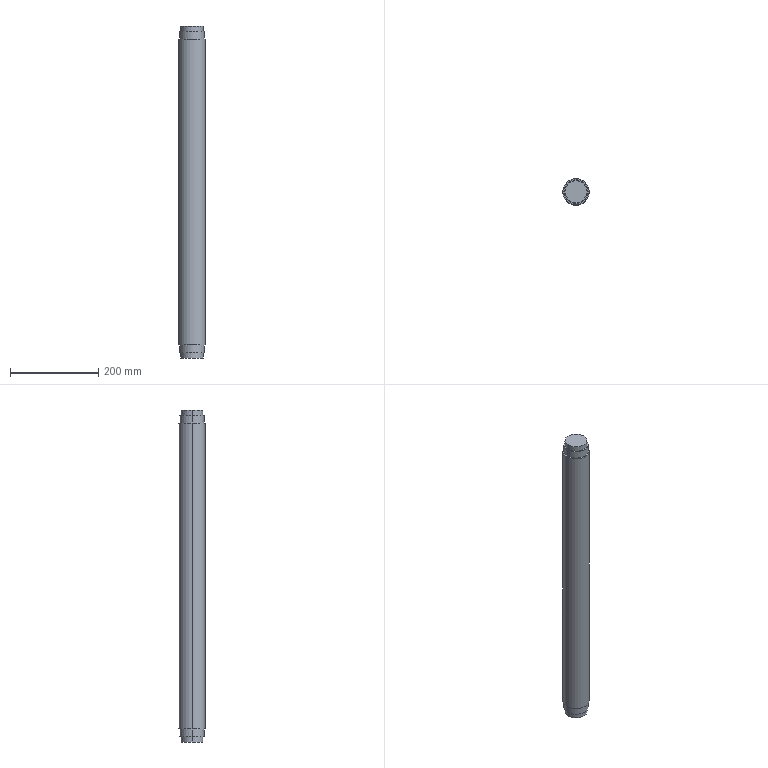Part | SolidWorks | features ICE 4, Extrusion 1 | 1 solid | 16 faces | box 60 x 60 x 754.2 mm | volume 2095819 mm3 | cylinder 10 | plane 6 | commonest cylinder face diameters 50 x4 55 x4 60 x2
STEP:
#1=CARTESIAN_POINT('',(25.,0.,742.2));
#2=VERTEX_POINT('',#1);
#3=CARTESIAN_POINT('',(-25.,0.,742.2));
#4=VERTEX_POINT('',#3);
#5=CARTESIAN_POINT('',(0.,0.,742.2));
#6=DIRECTION('',(0.,0.,1.));
#7=DIRECTION('',(1.,0.,0.));
#8=AXIS2_PLACEMENT_3D('',#5,#6,#7);
#9=CIRCLE('',#8,25.);
#10=EDGE_CURVE('',#2,#4,#9,.T.);
#11=ORIENTED_EDGE('',*,*,#10,.F.);
#12=CARTESIAN_POINT('',(25.,0.,730.2));
#13=VERTEX_POINT('',#12);
#14=CARTESIAN_POINT('',(25.,0.,742.2));
#15=DIRECTION('',(0.,0.,-1.));
#16=VECTOR('',#15,1000.);
#17=LINE('',#14,#16);
#18=EDGE_CURVE('',#2,#13,#17,.T.);
#19=ORIENTED_EDGE('',*,*,#18,.T.);
#20=CARTESIAN_POINT('',(-25.,0.,730.2));
#21=VERTEX_POINT('',#20);
#22=CARTESIAN_POINT('',(0.,0.,730.2));
#23=DIRECTION('',(0.,0.,1.));
#24=DIRECTION('',(1.,0.,0.));
#25=AXIS2_PLACEMENT_3D('',#22,#23,#24);
#26=CIRCLE('',#25,25.);
#27=EDGE_CURVE('',#13,#21,#26,.T.);
#28=ORIENTED_EDGE('',*,*,#27,.T.);
#29=CARTESIAN_POINT('',(-25.,0.,742.2));
#30=DIRECTION('',(0.,0.,-1.));
#31=VECTOR('',#30,1000.);
#32=LINE('',#29,#31);
#33=EDGE_CURVE('',#4,#21,#32,.T.);
#34=ORIENTED_EDGE('',*,*,#33,.F.);
#35=EDGE_LOOP('',(#11,#19,#28,#34));
#36=FACE_OUTER_BOUND('',#35,.T.);
#37=CARTESIAN_POINT('',(0.,0.,742.2));
#38=DIRECTION('',(0.,0.,-1.));
#39=DIRECTION('',(-1.,0.,0.));
#40=AXIS2_PLACEMENT_3D('',#37,#38,#39);
#41=CYLINDRICAL_SURFACE('',#40,25.);
#42=ADVANCED_FACE('',(#36),#41,.T.);
#43=CARTESIAN_POINT('',(27.5,0.,730.2));
#44=VERTEX_POINT('',#43);
#45=CARTESIAN_POINT('',(-27.5,0.,730.2));
#46=VERTEX_POINT('',#45);
#47=CARTESIAN_POINT('',(0.,0.,730.2));
#48=DIRECTION('',(0.,0.,1.));
#49=DIRECTION('',(1.,0.,0.));
#50=AXIS2_PLACEMENT_3D('',#47,#48,#49);
#51=CIRCLE('',#50,27.5);
#52=EDGE_CURVE('',#44,#46,#51,.T.);
#53=ORIENTED_EDGE('',*,*,#52,.F.);
#54=CARTESIAN_POINT('',(27.5,0.,712.6));
#55=VERTEX_POINT('',#54);
#56=CARTESIAN_POINT('',(27.5,0.,730.2));
#57=DIRECTION('',(0.,0.,-1.));
#58=VECTOR('',#57,1000.);
#59=LINE('',#56,#58);
#60=EDGE_CURVE('',#44,#55,#59,.T.);
#61=ORIENTED_EDGE('',*,*,#60,.T.);
#62=CARTESIAN_POINT('',(-27.5,0.,712.6));
#63=VERTEX_POINT('',#62);
#64=CARTESIAN_POINT('',(0.,0.,712.6));
#65=DIRECTION('',(0.,0.,1.));
#66=DIRECTION('',(1.,0.,0.));
#67=AXIS2_PLACEMENT_3D('',#64,#65,#66);
#68=CIRCLE('',#67,27.5);
#69=EDGE_CURVE('',#55,#63,#68,.T.);
#70=ORIENTED_EDGE('',*,*,#69,.T.);
#71=CARTESIAN_POINT('',(-27.5,0.,730.2));
#72=DIRECTION('',(0.,0.,-1.));
#73=VECTOR('',#72,1000.);
#74=LINE('',#71,#73);
#75=EDGE_CURVE('',#46,#63,#74,.T.);
#76=ORIENTED_EDGE('',*,*,#75,.F.);
#77=EDGE_LOOP('',(#53,#61,#70,#76));
#78=FACE_OUTER_BOUND('',#77,.T.);
#79=CARTESIAN_POINT('',(0.,0.,730.2));
#80=DIRECTION('',(0.,0.,-1.));
#81=DIRECTION('',(-1.,0.,0.));
#82=AXIS2_PLACEMENT_3D('',#79,#80,#81);
#83=CYLINDRICAL_SURFACE('',#82,27.5);
#84=ADVANCED_FACE('',(#78),#83,.T.);
#85=CARTESIAN_POINT('',(30.,0.,712.6));
#86=VERTEX_POINT('',#85);
#87=CARTESIAN_POINT('',(-30.,0.,712.6));
#88=VERTEX_POINT('',#87);
#89=CARTESIAN_POINT('',(0.,0.,712.6));
#90=DIRECTION('',(0.,0.,1.));
#91=DIRECTION('',(1.,0.,0.));
#92=AXIS2_PLACEMENT_3D('',#89,#90,#91);
#93=CIRCLE('',#92,30.);
#94=EDGE_CURVE('',#86,#88,#93,.T.);
#95=ORIENTED_EDGE('',*,*,#94,.F.);
#96=CARTESIAN_POINT('',(30.,0.,17.6));
#97=VERTEX_POINT('',#96);
#98=CARTESIAN_POINT('',(30.,0.,712.6));
#99=DIRECTION('',(0.,0.,-1.));
#100=VECTOR('',#99,1000.);
#101=LINE('',#98,#100);
#102=EDGE_CURVE('',#86,#97,#101,.T.);
#103=ORIENTED_EDGE('',*,*,#102,.T.);
#104=CARTESIAN_POINT('',(-30.,0.,17.6));
#105=VERTEX_POINT('',#104);
#106=CARTESIAN_POINT('',(0.,0.,17.6));
#107=DIRECTION('',(0.,0.,1.));
#108=DIRECTION('',(1.,0.,0.));
#109=AXIS2_PLACEMENT_3D('',#106,#107,#108);
#110=CIRCLE('',#109,30.);
#111=EDGE_CURVE('',#97,#105,#110,.T.);
#112=ORIENTED_EDGE('',*,*,#111,.T.);
#113=CARTESIAN_POINT('',(-30.,0.,712.6));
#114=DIRECTION('',(0.,0.,-1.));
#115=VECTOR('',#114,1000.);
#116=LINE('',#113,#115);
#117=EDGE_CURVE('',#88,#105,#116,.T.);
#118=ORIENTED_EDGE('',*,*,#117,.F.);
#119=EDGE_LOOP('',(#95,#103,#112,#118));
#120=FACE_OUTER_BOUND('',#119,.T.);
#121=CARTESIAN_POINT('',(0.,0.,712.6));
#122=DIRECTION('',(0.,0.,-1.));
#123=DIRECTION('',(-1.,0.,0.));
#124=AXIS2_PLACEMENT_3D('',#121,#122,#123);
#125=CYLINDRICAL_SURFACE('',#124,30.);
#126=ADVANCED_FACE('',(#120),#125,.T.);
#127=CARTESIAN_POINT('',(-25.,0.,-12.));
#128=VERTEX_POINT('',#127);
#129=CARTESIAN_POINT('',(25.,0.,-12.));
#130=VERTEX_POINT('',#129);
#131=CARTESIAN_POINT('',(0.,0.,-12.));
#132=DIRECTION('',(0.,0.,-1.));
#133=DIRECTION('',(-1.,0.,0.));
#134=AXIS2_PLACEMENT_3D('',#131,#132,#133);
#135=CIRCLE('',#134,25.);
#136=EDGE_CURVE('',#128,#130,#135,.T.);
#137=ORIENTED_EDGE('',*,*,#136,.F.);
#138=CARTESIAN_POINT('',(-25.,0.,0.));
#139=VERTEX_POINT('',#138);
#140=CARTESIAN_POINT('',(-25.,0.,-12.));
#141=DIRECTION('',(0.,0.,1.));
#142=VECTOR('',#141,1000.);
#143=LINE('',#140,#142);
#144=EDGE_CURVE('',#128,#139,#143,.T.);
#145=ORIENTED_EDGE('',*,*,#144,.T.);
#146=CARTESIAN_POINT('',(25.,0.,0.));
#147=VERTEX_POINT('',#146);
#148=CARTESIAN_POINT('',(0.,0.,0.));
#149=DIRECTION('',(0.,0.,-1.));
#150=DIRECTION('',(1.,0.,0.));
#151=AXIS2_PLACEMENT_3D('',#148,#149,#150);
#152=CIRCLE('',#151,25.);
#153=EDGE_CURVE('',#139,#147,#152,.T.);
#154=ORIENTED_EDGE('',*,*,#153,.T.);
#155=CARTESIAN_POINT('',(25.,0.,-12.));
#156=DIRECTION('',(0.,0.,1.));
#157=VECTOR('',#156,1000.);
#158=LINE('',#155,#157);
#159=EDGE_CURVE('',#130,#147,#158,.T.);
#160=ORIENTED_EDGE('',*,*,#159,.F.);
#161=EDGE_LOOP('',(#137,#145,#154,#160));
#162=FACE_OUTER_BOUND('',#161,.T.);
#163=CARTESIAN_POINT('',(0.,0.,-12.));
#164=DIRECTION('',(0.,0.,1.));
#165=DIRECTION('',(1.,0.,0.));
#166=AXIS2_PLACEMENT_3D('',#163,#164,#165);
#167=CYLINDRICAL_SURFACE('',#166,25.);
#168=ADVANCED_FACE('',(#162),#167,.T.);
#169=CARTESIAN_POINT('',(27.5,0.,17.6));
#170=VERTEX_POINT('',#169);
#171=CARTESIAN_POINT('',(-27.5,0.,17.6));
#172=VERTEX_POINT('',#171);
#173=CARTESIAN_POINT('',(0.,0.,17.6));
#174=DIRECTION('',(0.,0.,1.));
#175=DIRECTION('',(1.,0.,0.));
#176=AXIS2_PLACEMENT_3D('',#173,#174,#175);
#177=CIRCLE('',#176,27.5);
#178=EDGE_CURVE('',#170,#172,#177,.T.);
#179=ORIENTED_EDGE('',*,*,#178,.F.);
#180=CARTESIAN_POINT('',(27.5,0.,0.));
#181=VERTEX_POINT('',#180);
#182=CARTESIAN_POINT('',(27.5,0.,17.6));
#183=DIRECTION('',(0.,0.,-1.));
#184=VECTOR('',#183,1000.);
#185=LINE('',#182,#184);
#186=EDGE_CURVE('',#170,#181,#185,.T.);
#187=ORIENTED_EDGE('',*,*,#186,.T.);
#188=CARTESIAN_POINT('',(-27.5,0.,0.));
#189=VERTEX_POINT('',#188);
#190=CARTESIAN_POINT('',(0.,0.,0.));
#191=DIRECTION('',(0.,0.,1.));
#192=DIRECTION('',(1.,0.,0.));
#193=AXIS2_PLACEMENT_3D('',#190,#191,#192);
#194=CIRCLE('',#193,27.5);
#195=EDGE_CURVE('',#181,#189,#194,.T.);
#196=ORIENTED_EDGE('',*,*,#195,.T.);
#197=CARTESIAN_POINT('',(-27.5,0.,17.6));
#198=DIRECTION('',(0.,0.,-1.));
#199=VECTOR('',#198,1000.);
#200=LINE('',#197,#199);
#201=EDGE_CURVE('',#172,#189,#200,.T.);
#202=ORIENTED_EDGE('',*,*,#201,.F.);
#203=EDGE_LOOP('',(#179,#187,#196,#202));
#204=FACE_OUTER_BOUND('',#203,.T.);
#205=CARTESIAN_POINT('',(0.,0.,17.6));
#206=DIRECTION('',(0.,0.,-1.));
#207=DIRECTION('',(-1.,0.,0.));
#208=AXIS2_PLACEMENT_3D('',#205,#206,#207);
#209=CYLINDRICAL_SURFACE('',#208,27.5);
#210=ADVANCED_FACE('',(#204),#209,.T.);
#211=CARTESIAN_POINT('',(0.,0.,730.2));
#212=DIRECTION('',(0.,0.,1.));
#213=DIRECTION('',(1.,0.,0.));
#214=AXIS2_PLACEMENT_3D('',#211,#212,#213);
#215=CIRCLE('',#214,27.5);
#216=EDGE_CURVE('',#46,#44,#215,.T.);
#217=ORIENTED_EDGE('',*,*,#216,.T.);
#218=ORIENTED_EDGE('',*,*,#52,.T.);
#219=EDGE_LOOP('',(#217,#218));
#220=FACE_OUTER_BOUND('',#219,.T.);
#221=CARTESIAN_POINT('',(0.,0.,730.2));
#222=DIRECTION('',(0.,0.,1.));
#223=DIRECTION('',(1.,0.,0.));
#224=AXIS2_PLACEMENT_3D('',#221,#222,#223);
#225=CIRCLE('',#224,25.);
#226=EDGE_CURVE('',#21,#13,#225,.T.);
#227=ORIENTED_EDGE('',*,*,#226,.F.);
#228=ORIENTED_EDGE('',*,*,#27,.F.);
#229=EDGE_LOOP('',(#227,#228));
#230=FACE_BOUND('',#229,.T.);
#231=CARTESIAN_POINT('',(0.,0.,730.2));
#232=DIRECTION('',(0.,0.,1.));
#233=DIRECTION('',(1.,0.,0.));
#234=AXIS2_PLACEMENT_3D('',#231,#232,#233);
#235=PLANE('',#234);
#236=ADVANCED_FACE('',(#220,#230),#235,.T.);
#237=CARTESIAN_POINT('',(0.,0.,712.6));
#238=DIRECTION('',(0.,0.,1.));
#239=DIRECTION('',(1.,0.,0.));
#240=AXIS2_PLACEMENT_3D('',#237,#238,#239);
#241=CIRCLE('',#240,30.);
#242=EDGE_CURVE('',#88,#86,#241,.T.);
#243=ORIENTED_EDGE('',*,*,#242,.T.);
#244=ORIENTED_EDGE('',*,*,#94,.T.);
#245=EDGE_LOOP('',(#243,#244));
#246=FACE_OUTER_BOUND('',#245,.T.);
#247=CARTESIAN_POINT('',(0.,0.,712.6));
#248=DIRECTION('',(0.,0.,1.));
#249=DIRECTION('',(1.,0.,0.));
#250=AXIS2_PLACEMENT_3D('',#247,#248,#249);
#251=CIRCLE('',#250,27.5);
#252=EDGE_CURVE('',#63,#55,#251,.T.);
#253=ORIENTED_EDGE('',*,*,#252,.F.);
#254=ORIENTED_EDGE('',*,*,#69,.F.);
#255=EDGE_LOOP('',(#253,#254));
#256=FACE_BOUND('',#255,.T.);
#257=CARTESIAN_POINT('',(0.,0.,712.6));
#258=DIRECTION('',(0.,0.,1.));
#259=DIRECTION('',(1.,0.,0.));
#260=AXIS2_PLACEMENT_3D('',#257,#258,#259);
#261=PLANE('',#260);
#262=ADVANCED_FACE('',(#246,#256),#261,.T.);
#263=CARTESIAN_POINT('',(0.,0.,0.));
#264=DIRECTION('',(0.,0.,1.));
#265=DIRECTION('',(1.,0.,0.));
#266=AXIS2_PLACEMENT_3D('',#263,#264,#265);
#267=CIRCLE('',#266,27.5);
#268=EDGE_CURVE('',#189,#181,#267,.T.);
#269=ORIENTED_EDGE('',*,*,#268,.F.);
#270=ORIENTED_EDGE('',*,*,#195,.F.);
#271=EDGE_LOOP('',(#269,#270));
#272=FACE_OUTER_BOUND('',#271,.T.);
#273=CARTESIAN_POINT('',(0.,0.,0.));
#274=DIRECTION('',(0.,0.,-1.));
#275=DIRECTION('',(1.,0.,0.));
#276=AXIS2_PLACEMENT_3D('',#273,#274,#275);
#277=CIRCLE('',#276,25.);
#278=EDGE_CURVE('',#147,#139,#277,.T.);
#279=ORIENTED_EDGE('',*,*,#278,.F.);
#280=ORIENTED_EDGE('',*,*,#153,.F.);
#281=EDGE_LOOP('',(#279,#280));
#282=FACE_BOUND('',#281,.T.);
#283=CARTESIAN_POINT('',(0.,0.,0.));
#284=DIRECTION('',(0.,0.,1.));
#285=DIRECTION('',(1.,0.,0.));
#286=AXIS2_PLACEMENT_3D('',#283,#284,#285);
#287=PLANE('',#286);
#288=ADVANCED_FACE('',(#272,#282),#287,.F.);
#289=ORIENTED_EDGE('',*,*,#186,.F.);
#290=CARTESIAN_POINT('',(0.,0.,17.6));
#291=DIRECTION('',(0.,0.,1.));
#292=DIRECTION('',(1.,0.,0.));
#293=AXIS2_PLACEMENT_3D('',#290,#291,#292);
#294=CIRCLE('',#293,27.5);
#295=EDGE_CURVE('',#172,#170,#294,.T.);
#296=ORIENTED_EDGE('',*,*,#295,.F.);
#297=ORIENTED_EDGE('',*,*,#201,.T.);
#298=ORIENTED_EDGE('',*,*,#268,.T.);
#299=EDGE_LOOP('',(#289,#296,#297,#298));
#300=FACE_OUTER_BOUND('',#299,.T.);
#301=CARTESIAN_POINT('',(0.,0.,17.6));
#302=DIRECTION('',(0.,0.,-1.));
#303=DIRECTION('',(-1.,0.,0.));
#304=AXIS2_PLACEMENT_3D('',#301,#302,#303);
#305=CYLINDRICAL_SURFACE('',#304,27.5);
#306=ADVANCED_FACE('',(#300),#305,.T.);
#307=ORIENTED_EDGE('',*,*,#144,.F.);
#308=CARTESIAN_POINT('',(0.,0.,-12.));
#309=DIRECTION('',(0.,0.,-1.));
#310=DIRECTION('',(-1.,0.,0.));
#311=AXIS2_PLACEMENT_3D('',#308,#309,#310);
#312=CIRCLE('',#311,25.);
#313=EDGE_CURVE('',#130,#128,#312,.T.);
#314=ORIENTED_EDGE('',*,*,#313,.F.);
#315=ORIENTED_EDGE('',*,*,#159,.T.);
#316=ORIENTED_EDGE('',*,*,#278,.T.);
#317=EDGE_LOOP('',(#307,#314,#315,#316));
#318=FACE_OUTER_BOUND('',#317,.T.);
#319=CARTESIAN_POINT('',(0.,0.,-12.));
#320=DIRECTION('',(0.,0.,1.));
#321=DIRECTION('',(1.,0.,0.));
#322=AXIS2_PLACEMENT_3D('',#319,#320,#321);
#323=CYLINDRICAL_SURFACE('',#322,25.);
#324=ADVANCED_FACE('',(#318),#323,.T.);
#325=ORIENTED_EDGE('',*,*,#313,.T.);
#326=ORIENTED_EDGE('',*,*,#136,.T.);
#327=EDGE_LOOP('',(#325,#326));
#328=FACE_OUTER_BOUND('',#327,.T.);
#329=CARTESIAN_POINT('',(0.,0.,-12.));
#330=DIRECTION('',(0.,0.,-1.));
#331=DIRECTION('',(-1.,0.,0.));
#332=AXIS2_PLACEMENT_3D('',#329,#330,#331);
#333=PLANE('',#332);
#334=ADVANCED_FACE('',(#328),#333,.T.);
#335=CARTESIAN_POINT('',(0.,0.,17.6));
#336=DIRECTION('',(0.,0.,1.));
#337=DIRECTION('',(1.,0.,0.));
#338=AXIS2_PLACEMENT_3D('',#335,#336,#337);
#339=CIRCLE('',#338,30.);
#340=EDGE_CURVE('',#105,#97,#339,.T.);
#341=ORIENTED_EDGE('',*,*,#340,.F.);
#342=ORIENTED_EDGE('',*,*,#111,.F.);
#343=EDGE_LOOP('',(#341,#342));
#344=FACE_OUTER_BOUND('',#343,.T.);
#345=ORIENTED_EDGE('',*,*,#295,.T.);
#346=ORIENTED_EDGE('',*,*,#178,.T.);
#347=EDGE_LOOP('',(#345,#346));
#348=FACE_BOUND('',#347,.T.);
#349=CARTESIAN_POINT('',(0.,0.,17.6));
#350=DIRECTION('',(0.,0.,1.));
#351=DIRECTION('',(1.,0.,0.));
#352=AXIS2_PLACEMENT_3D('',#349,#350,#351);
#353=PLANE('',#352);
#354=ADVANCED_FACE('',(#344,#348),#353,.F.);
#355=ORIENTED_EDGE('',*,*,#102,.F.);
#356=ORIENTED_EDGE('',*,*,#242,.F.);
#357=ORIENTED_EDGE('',*,*,#117,.T.);
#358=ORIENTED_EDGE('',*,*,#340,.T.);
#359=EDGE_LOOP('',(#355,#356,#357,#358));
#360=FACE_OUTER_BOUND('',#359,.T.);
#361=CARTESIAN_POINT('',(0.,0.,712.6));
#362=DIRECTION('',(0.,0.,-1.));
#363=DIRECTION('',(-1.,0.,0.));
#364=AXIS2_PLACEMENT_3D('',#361,#362,#363);
#365=CYLINDRICAL_SURFACE('',#364,30.);
#366=ADVANCED_FACE('',(#360),#365,.T.);
#367=ORIENTED_EDGE('',*,*,#60,.F.);
#368=ORIENTED_EDGE('',*,*,#216,.F.);
#369=ORIENTED_EDGE('',*,*,#75,.T.);
#370=ORIENTED_EDGE('',*,*,#252,.T.);
#371=EDGE_LOOP('',(#367,#368,#369,#370));
#372=FACE_OUTER_BOUND('',#371,.T.);
#373=CARTESIAN_POINT('',(0.,0.,730.2));
#374=DIRECTION('',(0.,0.,-1.));
#375=DIRECTION('',(-1.,0.,0.));
#376=AXIS2_PLACEMENT_3D('',#373,#374,#375);
#377=CYLINDRICAL_SURFACE('',#376,27.5);
#378=ADVANCED_FACE('',(#372),#377,.T.);
#379=ORIENTED_EDGE('',*,*,#18,.F.);
#380=CARTESIAN_POINT('',(0.,0.,742.2));
#381=DIRECTION('',(0.,0.,1.));
#382=DIRECTION('',(1.,0.,0.));
#383=AXIS2_PLACEMENT_3D('',#380,#381,#382);
#384=CIRCLE('',#383,25.);
#385=EDGE_CURVE('',#4,#2,#384,.T.);
#386=ORIENTED_EDGE('',*,*,#385,.F.);
#387=ORIENTED_EDGE('',*,*,#33,.T.);
#388=ORIENTED_EDGE('',*,*,#226,.T.);
#389=EDGE_LOOP('',(#379,#386,#387,#388));
#390=FACE_OUTER_BOUND('',#389,.T.);
#391=CARTESIAN_POINT('',(0.,0.,742.2));
#392=DIRECTION('',(0.,0.,-1.));
#393=DIRECTION('',(-1.,0.,0.));
#394=AXIS2_PLACEMENT_3D('',#391,#392,#393);
#395=CYLINDRICAL_SURFACE('',#394,25.);
#396=ADVANCED_FACE('',(#390),#395,.T.);
#397=ORIENTED_EDGE('',*,*,#385,.T.);
#398=ORIENTED_EDGE('',*,*,#10,.T.);
#399=EDGE_LOOP('',(#397,#398));
#400=FACE_OUTER_BOUND('',#399,.T.);
#401=CARTESIAN_POINT('',(0.,0.,742.2));
#402=DIRECTION('',(0.,0.,1.));
#403=DIRECTION('',(1.,0.,0.));
#404=AXIS2_PLACEMENT_3D('',#401,#402,#403);
#405=PLANE('',#404);
#406=ADVANCED_FACE('',(#400),#405,.T.);
#407=CLOSED_SHELL('',(#42,#84,#126,#168,#210,#236,#262,#288,#306,#324,#334,#354,#366,#378,#396,#406));
#408=MANIFOLD_SOLID_BREP('',#407);
#409=CARTESIAN_POINT('',(0.,0.,0.));
#410=DIRECTION('',(0.,0.,1.));
#411=DIRECTION('',(1.,0.,0.));
#412=AXIS2_PLACEMENT_3D('',#409,#410,#411);
#413=(LENGTH_UNIT()NAMED_UNIT(*)SI_UNIT(.MILLI.,.METRE.));
#414=UNCERTAINTY_MEASURE_WITH_UNIT(LENGTH_MEASURE(0.00001),#413,'','');
#415=(NAMED_UNIT(*)PLANE_ANGLE_UNIT()SI_UNIT($,.RADIAN.));
#416=(NAMED_UNIT(*)SI_UNIT($,.STERADIAN.)SOLID_ANGLE_UNIT());
#417=(GEOMETRIC_REPRESENTATION_CONTEXT(3)GLOBAL_UNCERTAINTY_ASSIGNED_CONTEXT((#414))GLOBAL_UNIT_ASSIGNED_CONTEXT((#413,#415,#416))REPRESENTATION_CONTEXT('',''));
#418=ADVANCED_BREP_SHAPE_REPRESENTATION('',(#408,#412),#417);